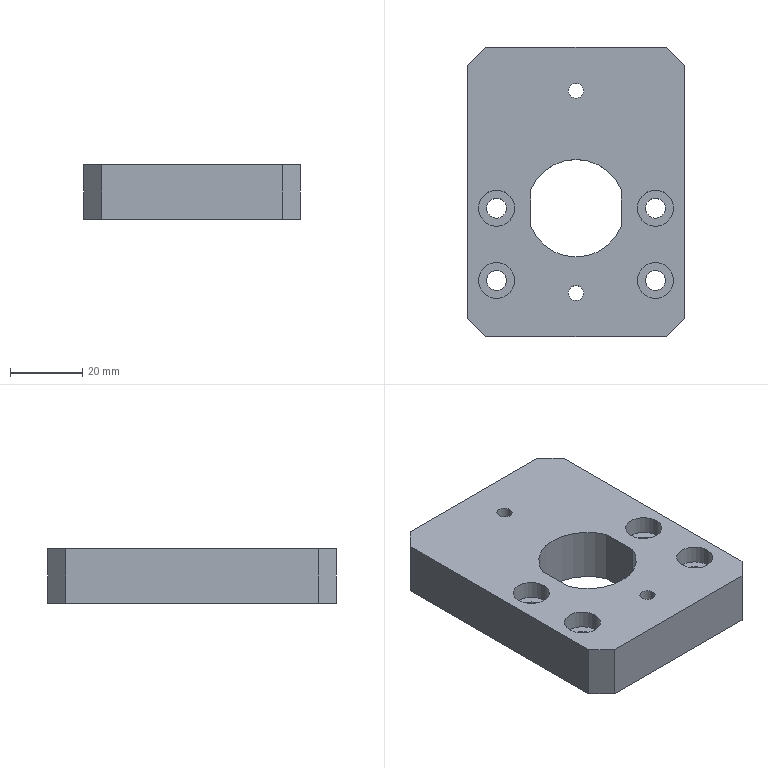Part | STEP file | slingshot detection positioning | 1 solid | 38 faces | box 60 x 80 x 15 mm | volume 59930 mm3 | cylinder 22 | plane 16 | commonest cylinder face diameters 5.5 x8 10 x8 4.2 x4 27 x2